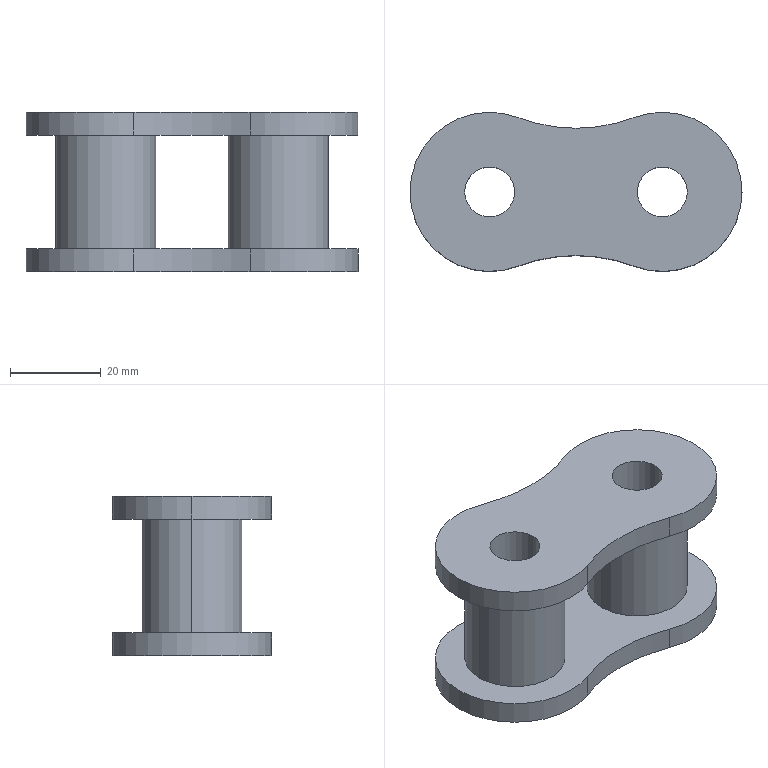Part | STEP file | 24A double-side double-hole chain 2 | 1 solid | 22 faces | box 73 x 35 x 35 mm | volume 33789 mm3 | cylinder 18 | plane 4 | commonest cylinder face diameters 35 x6 11 x4 22 x4 71.643 x4